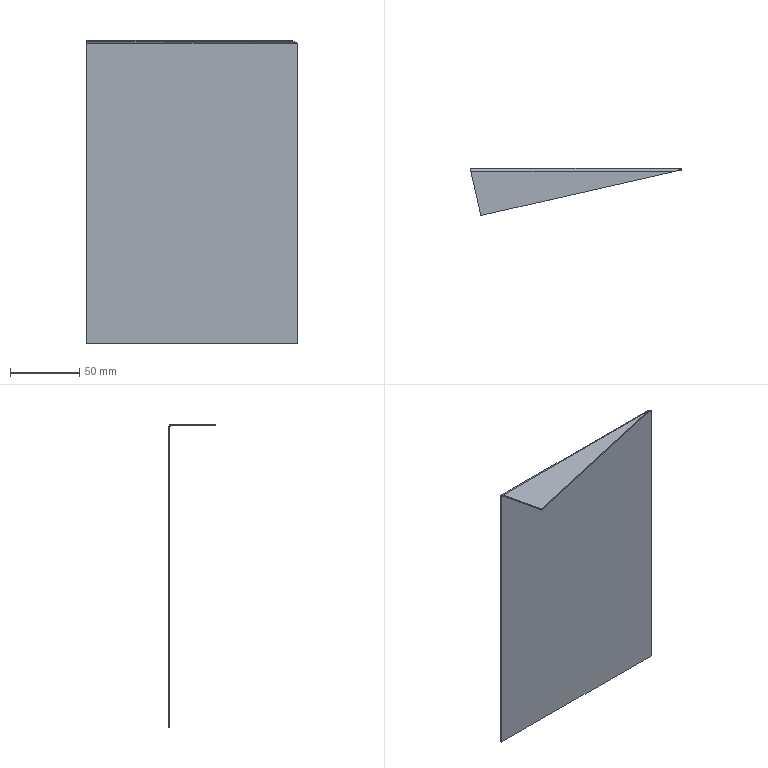Part | 1 solid | 13 faces | box 152.5 x 34 x 219 mm | volume 35812 mm3 | plane 9 | spline 2 | cylinder 2 | commonest cylinder face diameters 2 x1 4 x1
STEP:
#1=CARTESIAN_POINT('',(-152.5,-1.,107.5));
#2=VERTEX_POINT('',#1);
#3=CARTESIAN_POINT('',(0.,-1.,107.5));
#4=VERTEX_POINT('',#3);
#5=CARTESIAN_POINT('',(-152.5,-1.,107.5));
#6=DIRECTION('',(1.,0.,0.));
#7=VECTOR('',#6,1000.);
#8=LINE('',#5,#7);
#9=EDGE_CURVE('',#2,#4,#8,.T.);
#10=ORIENTED_EDGE('',*,*,#9,.F.);
#11=CARTESIAN_POINT('',(-152.5,-1.,-109.5));
#12=VERTEX_POINT('',#11);
#13=CARTESIAN_POINT('',(-152.5,-1.,109.5));
#14=DIRECTION('',(0.,0.,-1.));
#15=VECTOR('',#14,1000.);
#16=LINE('',#13,#15);
#17=EDGE_CURVE('',#2,#12,#16,.T.);
#18=ORIENTED_EDGE('',*,*,#17,.T.);
#19=CARTESIAN_POINT('',(0.,-1.,-109.5));
#20=VERTEX_POINT('',#19);
#21=CARTESIAN_POINT('',(-152.5,-1.,-109.5));
#22=DIRECTION('',(1.,0.,0.));
#23=VECTOR('',#22,1000.);
#24=LINE('',#21,#23);
#25=EDGE_CURVE('',#12,#20,#24,.T.);
#26=ORIENTED_EDGE('',*,*,#25,.T.);
#27=CARTESIAN_POINT('',(0.,-1.,109.5));
#28=DIRECTION('',(0.,0.,-1.));
#29=VECTOR('',#28,1000.);
#30=LINE('',#27,#29);
#31=EDGE_CURVE('',#4,#20,#30,.T.);
#32=ORIENTED_EDGE('',*,*,#31,.F.);
#33=EDGE_LOOP('',(#10,#18,#26,#32));
#34=FACE_OUTER_BOUND('',#33,.T.);
#35=CARTESIAN_POINT('',(-152.5,-1.,109.5));
#36=DIRECTION('',(0.,1.,0.));
#37=DIRECTION('',(0.,0.,1.));
#38=AXIS2_PLACEMENT_3D('',#35,#36,#37);
#39=PLANE('',#38);
#40=ADVANCED_FACE('',(#34),#39,.F.);
#41=CARTESIAN_POINT('',(-152.5,0.,107.5));
#42=VERTEX_POINT('',#41);
#43=CARTESIAN_POINT('',(-152.5,0.,-109.5));
#44=VERTEX_POINT('',#43);
#45=CARTESIAN_POINT('',(-152.5,0.,109.5));
#46=DIRECTION('',(0.,0.,-1.));
#47=VECTOR('',#46,1000.);
#48=LINE('',#45,#47);
#49=EDGE_CURVE('',#42,#44,#48,.T.);
#50=ORIENTED_EDGE('',*,*,#49,.F.);
#51=CARTESIAN_POINT('',(0.,0.,107.5));
#52=VERTEX_POINT('',#51);
#53=CARTESIAN_POINT('',(-152.5,0.,107.5));
#54=DIRECTION('',(1.,0.,0.));
#55=VECTOR('',#54,1000.);
#56=LINE('',#53,#55);
#57=EDGE_CURVE('',#42,#52,#56,.T.);
#58=ORIENTED_EDGE('',*,*,#57,.T.);
#59=CARTESIAN_POINT('',(0.,0.,-109.5));
#60=VERTEX_POINT('',#59);
#61=CARTESIAN_POINT('',(0.,0.,109.5));
#62=DIRECTION('',(0.,0.,-1.));
#63=VECTOR('',#62,1000.);
#64=LINE('',#61,#63);
#65=EDGE_CURVE('',#52,#60,#64,.T.);
#66=ORIENTED_EDGE('',*,*,#65,.T.);
#67=CARTESIAN_POINT('',(-152.5,0.,-109.5));
#68=DIRECTION('',(1.,0.,0.));
#69=VECTOR('',#68,1000.);
#70=LINE('',#67,#69);
#71=EDGE_CURVE('',#44,#60,#70,.T.);
#72=ORIENTED_EDGE('',*,*,#71,.F.);
#73=EDGE_LOOP('',(#50,#58,#66,#72));
#74=FACE_OUTER_BOUND('',#73,.T.);
#75=CARTESIAN_POINT('',(-152.5,0.,109.5));
#76=DIRECTION('',(0.,1.,0.));
#77=DIRECTION('',(0.,0.,1.));
#78=AXIS2_PLACEMENT_3D('',#75,#76,#77);
#79=PLANE('',#78);
#80=ADVANCED_FACE('',(#74),#79,.T.);
#81=ORIENTED_EDGE('',*,*,#17,.F.);
#82=CARTESIAN_POINT('',(-152.5,-1.,107.5));
#83=DIRECTION('',(0.,1.,0.));
#84=VECTOR('',#83,1000.);
#85=LINE('',#82,#84);
#86=EDGE_CURVE('',#2,#42,#85,.T.);
#87=ORIENTED_EDGE('',*,*,#86,.T.);
#88=ORIENTED_EDGE('',*,*,#49,.T.);
#89=CARTESIAN_POINT('',(-152.5,-1.,-109.5));
#90=DIRECTION('',(0.,1.,0.));
#91=VECTOR('',#90,1000.);
#92=LINE('',#89,#91);
#93=EDGE_CURVE('',#12,#44,#92,.T.);
#94=ORIENTED_EDGE('',*,*,#93,.F.);
#95=EDGE_LOOP('',(#81,#87,#88,#94));
#96=FACE_OUTER_BOUND('',#95,.T.);
#97=CARTESIAN_POINT('',(-152.5,-1.,109.5));
#98=DIRECTION('',(-1.,0.,0.));
#99=DIRECTION('',(0.,0.,1.));
#100=AXIS2_PLACEMENT_3D('',#97,#98,#99);
#101=PLANE('',#100);
#102=ADVANCED_FACE('',(#96),#101,.T.);
#103=CARTESIAN_POINT('',(0.,-1.,107.5));
#104=DIRECTION('',(0.,1.,0.));
#105=VECTOR('',#104,1000.);
#106=LINE('',#103,#105);
#107=EDGE_CURVE('',#4,#52,#106,.T.);
#108=ORIENTED_EDGE('',*,*,#107,.F.);
#109=ORIENTED_EDGE('',*,*,#31,.T.);
#110=CARTESIAN_POINT('',(0.,0.,-109.5));
#111=DIRECTION('',(0.,-1.,0.));
#112=VECTOR('',#111,1000.);
#113=LINE('',#110,#112);
#114=EDGE_CURVE('',#60,#20,#113,.T.);
#115=ORIENTED_EDGE('',*,*,#114,.F.);
#116=ORIENTED_EDGE('',*,*,#65,.F.);
#117=EDGE_LOOP('',(#108,#109,#115,#116));
#118=FACE_OUTER_BOUND('',#117,.T.);
#119=CARTESIAN_POINT('',(0.,0.,109.5));
#120=DIRECTION('',(1.,0.,0.));
#121=DIRECTION('',(0.,0.,-1.));
#122=AXIS2_PLACEMENT_3D('',#119,#120,#121);
#123=PLANE('',#122);
#124=ADVANCED_FACE('',(#118),#123,.T.);
#125=ORIENTED_EDGE('',*,*,#25,.F.);
#126=ORIENTED_EDGE('',*,*,#93,.T.);
#127=ORIENTED_EDGE('',*,*,#71,.T.);
#128=ORIENTED_EDGE('',*,*,#114,.T.);
#129=EDGE_LOOP('',(#125,#126,#127,#128));
#130=FACE_OUTER_BOUND('',#129,.T.);
#131=CARTESIAN_POINT('',(0.,0.,-109.5));
#132=DIRECTION('',(0.,0.,-1.));
#133=DIRECTION('',(-1.,0.,0.));
#134=AXIS2_PLACEMENT_3D('',#131,#132,#133);
#135=PLANE('',#134);
#136=ADVANCED_FACE('',(#130),#135,.T.);
#137=CARTESIAN_POINT('',(-4.394,-2.,108.5));
#138=VERTEX_POINT('',#137);
#139=CARTESIAN_POINT('',(-4.394,-2.,109.5));
#140=VERTEX_POINT('',#139);
#141=CARTESIAN_POINT('',(-4.394,-2.,109.5));
#142=DIRECTION('',(0.,0.,1.));
#143=VECTOR('',#142,1000.);
#144=LINE('',#141,#143);
#145=EDGE_CURVE('',#138,#140,#144,.T.);
#146=ORIENTED_EDGE('',*,*,#145,.F.);
#147=CARTESIAN_POINT('',(0.,-1.,107.5));
#148=CARTESIAN_POINT('',(-0.3672,-1.,107.631));
#149=CARTESIAN_POINT('',(-0.7317,-1.026,107.762));
#150=CARTESIAN_POINT('',(-1.462,-1.126,108.003));
#151=CARTESIAN_POINT('',(-1.828,-1.2,108.114));
#152=CARTESIAN_POINT('',(-2.561,-1.385,108.299));
#153=CARTESIAN_POINT('',(-2.928,-1.496,108.374));
#154=CARTESIAN_POINT('',(-3.661,-1.738,108.474));
#155=CARTESIAN_POINT('',(-4.026,-1.869,108.5));
#156=CARTESIAN_POINT('',(-4.394,-2.,108.5));
#157=B_SPLINE_CURVE_WITH_KNOTS('',3,(#147,#148,#149,#150,#151,#152,#153,#154,#155,#156),.UNSPECIFIED.,.F.,.F.,(4,2,2,2,4),(0.,0.001162,0.002325,0.003487,0.00465),.UNSPECIFIED.);
#158=EDGE_CURVE('',#4,#138,#157,.T.);
#159=ORIENTED_EDGE('',*,*,#158,.F.);
#160=ORIENTED_EDGE('',*,*,#107,.T.);
#161=CARTESIAN_POINT('',(0.,0.,107.5));
#162=CARTESIAN_POINT('',(-0.3691,0.,107.764));
#163=CARTESIAN_POINT('',(-0.7313,-0.052,108.023));
#164=CARTESIAN_POINT('',(-1.46,-0.2511,108.505));
#165=CARTESIAN_POINT('',(-1.831,-0.4008,108.729));
#166=CARTESIAN_POINT('',(-2.56,-0.7691,109.098));
#167=CARTESIAN_POINT('',(-2.923,-0.9887,109.246));
#168=CARTESIAN_POINT('',(-3.66,-1.476,109.448));
#169=CARTESIAN_POINT('',(-4.024,-1.736,109.5));
#170=CARTESIAN_POINT('',(-4.394,-2.,109.5));
#171=B_SPLINE_CURVE_WITH_KNOTS('',3,(#161,#162,#163,#164,#165,#166,#167,#168,#169,#170),.UNSPECIFIED.,.F.,.F.,(4,2,2,2,4),(0.,0.001342,0.002685,0.004027,0.005369),.UNSPECIFIED.);
#172=EDGE_CURVE('',#52,#140,#171,.T.);
#173=ORIENTED_EDGE('',*,*,#172,.T.);
#174=EDGE_LOOP('',(#146,#159,#160,#173));
#175=FACE_OUTER_BOUND('',#174,.T.);
#176=CARTESIAN_POINT('',(0.,0.01,107.5));
#177=CARTESIAN_POINT('',(-0.3662,0.01,107.763));
#178=CARTESIAN_POINT('',(-0.7323,-0.04231,108.026));
#179=CARTESIAN_POINT('',(-1.465,-0.2437,108.512));
#180=CARTESIAN_POINT('',(-1.831,-0.3927,108.735));
#181=CARTESIAN_POINT('',(-2.563,-0.7648,109.107));
#182=CARTESIAN_POINT('',(-2.929,-0.9877,109.256));
#183=CARTESIAN_POINT('',(-3.661,-1.474,109.458));
#184=CARTESIAN_POINT('',(-4.027,-1.737,109.51));
#185=CARTESIAN_POINT('',(-4.394,-2.,109.51));
#186=CARTESIAN_POINT('',(0.,0.,107.5));
#187=CARTESIAN_POINT('',(-0.3662,0.,107.762));
#188=CARTESIAN_POINT('',(-0.7323,-0.05205,108.023));
#189=CARTESIAN_POINT('',(-1.465,-0.2524,108.507));
#190=CARTESIAN_POINT('',(-1.831,-0.4007,108.729));
#191=CARTESIAN_POINT('',(-2.563,-0.7709,109.099));
#192=CARTESIAN_POINT('',(-2.929,-0.9928,109.248));
#193=CARTESIAN_POINT('',(-3.661,-1.477,109.448));
#194=CARTESIAN_POINT('',(-4.027,-1.738,109.5));
#195=CARTESIAN_POINT('',(-4.394,-2.,109.5));
#196=CARTESIAN_POINT('',(0.,-1.,107.5));
#197=CARTESIAN_POINT('',(-0.3661,-1.,107.631));
#198=CARTESIAN_POINT('',(-0.7323,-1.026,107.762));
#199=CARTESIAN_POINT('',(-1.465,-1.126,108.004));
#200=CARTESIAN_POINT('',(-1.831,-1.2,108.115));
#201=CARTESIAN_POINT('',(-2.563,-1.385,108.3));
#202=CARTESIAN_POINT('',(-2.929,-1.496,108.374));
#203=CARTESIAN_POINT('',(-3.661,-1.738,108.474));
#204=CARTESIAN_POINT('',(-4.027,-1.869,108.5));
#205=CARTESIAN_POINT('',(-4.394,-2.,108.5));
#206=CARTESIAN_POINT('',(0.,-1.01,107.5));
#207=CARTESIAN_POINT('',(-0.3661,-1.01,107.63));
#208=CARTESIAN_POINT('',(-0.7323,-1.036,107.759));
#209=CARTESIAN_POINT('',(-1.465,-1.135,107.999));
#210=CARTESIAN_POINT('',(-1.831,-1.208,108.108));
#211=CARTESIAN_POINT('',(-2.563,-1.392,108.292));
#212=CARTESIAN_POINT('',(-2.929,-1.501,108.365));
#213=CARTESIAN_POINT('',(-3.661,-1.741,108.464));
#214=CARTESIAN_POINT('',(-4.027,-1.87,108.49));
#215=CARTESIAN_POINT('',(-4.394,-2.,108.49));
#216=B_SPLINE_SURFACE_WITH_KNOTS('',1,3,((#176,#177,#178,#179,#180,#181,#182,#183,#184,#185),(#186,#187,#188,#189,#190,#191,#192,#193,#194,#195),(#196,#197,#198,#199,#200,#201,#202,#203,#204,#205),(#206,#207,#208,#209,#210,#211,#212,#213,#214,#215)),.UNSPECIFIED.,.F.,.F.,.F.,(2,1,1,2),(4,2,2,2,4),(-0.01,0.,1.,1.01),(0.,0.25,0.5,0.75,1.),.UNSPECIFIED.);
#217=ADVANCED_FACE('',(#175),#216,.F.);
#218=CARTESIAN_POINT('',(-152.272,-2.,108.5));
#219=VERTEX_POINT('',#218);
#220=CARTESIAN_POINT('',(-152.272,-2.,108.5));
#221=CARTESIAN_POINT('',(-152.31,-1.738,108.5));
#222=CARTESIAN_POINT('',(-152.348,-1.478,108.392));
#223=CARTESIAN_POINT('',(-152.424,-1.108,108.022));
#224=CARTESIAN_POINT('',(-152.462,-1.,107.762));
#225=CARTESIAN_POINT('',(-152.5,-1.,107.5));
#226=B_SPLINE_CURVE_WITH_KNOTS('',3,(#220,#221,#222,#223,#224,#225),.UNSPECIFIED.,.F.,.F.,(4,2,4),(0.,0.5,1.),.UNSPECIFIED.);
#227=EDGE_CURVE('',#219,#2,#226,.T.);
#228=ORIENTED_EDGE('',*,*,#227,.F.);
#229=CARTESIAN_POINT('',(-152.272,-2.,109.5));
#230=VERTEX_POINT('',#229);
#231=CARTESIAN_POINT('',(-152.272,-2.,108.5));
#232=DIRECTION('',(0.,0.,1.));
#233=VECTOR('',#232,1000.);
#234=LINE('',#231,#233);
#235=EDGE_CURVE('',#219,#230,#234,.T.);
#236=ORIENTED_EDGE('',*,*,#235,.T.);
#237=CARTESIAN_POINT('',(-152.272,-2.,109.5));
#238=CARTESIAN_POINT('',(-152.291,-1.738,109.5));
#239=CARTESIAN_POINT('',(-152.31,-1.477,109.448));
#240=CARTESIAN_POINT('',(-152.348,-0.9928,109.248));
#241=CARTESIAN_POINT('',(-152.367,-0.7709,109.099));
#242=CARTESIAN_POINT('',(-152.405,-0.4007,108.729));
#243=CARTESIAN_POINT('',(-152.424,-0.2524,108.507));
#244=CARTESIAN_POINT('',(-152.462,-0.05205,108.023));
#245=CARTESIAN_POINT('',(-152.481,0.,107.762));
#246=CARTESIAN_POINT('',(-152.5,0.,107.5));
#247=B_SPLINE_CURVE_WITH_KNOTS('',3,(#237,#238,#239,#240,#241,#242,#243,#244,#245,#246),.UNSPECIFIED.,.F.,.F.,(4,2,2,2,4),(0.,0.25,0.5,0.75,1.),.UNSPECIFIED.);
#248=EDGE_CURVE('',#230,#42,#247,.T.);
#249=ORIENTED_EDGE('',*,*,#248,.T.);
#250=ORIENTED_EDGE('',*,*,#86,.F.);
#251=EDGE_LOOP('',(#228,#236,#249,#250));
#252=FACE_OUTER_BOUND('',#251,.T.);
#253=CARTESIAN_POINT('',(-152.272,-2.,109.51));
#254=CARTESIAN_POINT('',(-152.291,-1.737,109.51));
#255=CARTESIAN_POINT('',(-152.31,-1.474,109.458));
#256=CARTESIAN_POINT('',(-152.348,-0.9877,109.256));
#257=CARTESIAN_POINT('',(-152.367,-0.7648,109.107));
#258=CARTESIAN_POINT('',(-152.405,-0.3927,108.735));
#259=CARTESIAN_POINT('',(-152.424,-0.2437,108.512));
#260=CARTESIAN_POINT('',(-152.462,-0.04231,108.026));
#261=CARTESIAN_POINT('',(-152.481,0.01,107.763));
#262=CARTESIAN_POINT('',(-152.5,0.01,107.5));
#263=CARTESIAN_POINT('',(-152.272,-2.,109.5));
#264=CARTESIAN_POINT('',(-152.291,-1.738,109.5));
#265=CARTESIAN_POINT('',(-152.31,-1.477,109.448));
#266=CARTESIAN_POINT('',(-152.348,-0.9928,109.248));
#267=CARTESIAN_POINT('',(-152.367,-0.7709,109.099));
#268=CARTESIAN_POINT('',(-152.405,-0.4007,108.729));
#269=CARTESIAN_POINT('',(-152.424,-0.2524,108.507));
#270=CARTESIAN_POINT('',(-152.462,-0.05205,108.023));
#271=CARTESIAN_POINT('',(-152.481,0.,107.762));
#272=CARTESIAN_POINT('',(-152.5,0.,107.5));
#273=CARTESIAN_POINT('',(-152.272,-2.,108.5));
#274=CARTESIAN_POINT('',(-152.291,-1.869,108.5));
#275=CARTESIAN_POINT('',(-152.31,-1.738,108.474));
#276=CARTESIAN_POINT('',(-152.348,-1.496,108.374));
#277=CARTESIAN_POINT('',(-152.367,-1.385,108.3));
#278=CARTESIAN_POINT('',(-152.405,-1.2,108.115));
#279=CARTESIAN_POINT('',(-152.424,-1.126,108.004));
#280=CARTESIAN_POINT('',(-152.462,-1.026,107.762));
#281=CARTESIAN_POINT('',(-152.481,-1.,107.631));
#282=CARTESIAN_POINT('',(-152.5,-1.,107.5));
#283=CARTESIAN_POINT('',(-152.272,-2.,108.49));
#284=CARTESIAN_POINT('',(-152.291,-1.87,108.49));
#285=CARTESIAN_POINT('',(-152.31,-1.741,108.464));
#286=CARTESIAN_POINT('',(-152.348,-1.501,108.365));
#287=CARTESIAN_POINT('',(-152.367,-1.392,108.292));
#288=CARTESIAN_POINT('',(-152.405,-1.208,108.108));
#289=CARTESIAN_POINT('',(-152.424,-1.135,107.999));
#290=CARTESIAN_POINT('',(-152.462,-1.036,107.759));
#291=CARTESIAN_POINT('',(-152.481,-1.01,107.63));
#292=CARTESIAN_POINT('',(-152.5,-1.01,107.5));
#293=B_SPLINE_SURFACE_WITH_KNOTS('',1,3,((#253,#254,#255,#256,#257,#258,#259,#260,#261,#262),(#263,#264,#265,#266,#267,#268,#269,#270,#271,#272),(#273,#274,#275,#276,#277,#278,#279,#280,#281,#282),(#283,#284,#285,#286,#287,#288,#289,#290,#291,#292)),.UNSPECIFIED.,.F.,.F.,.F.,(2,1,1,2),(4,2,2,2,4),(-0.01,0.,1.,1.01),(0.,0.25,0.5,0.75,1.),.UNSPECIFIED.);
#294=ADVANCED_FACE('',(#252),#293,.F.);
#295=ORIENTED_EDGE('',*,*,#57,.F.);
#296=ORIENTED_EDGE('',*,*,#248,.F.);
#297=CARTESIAN_POINT('',(0.,-2.,109.5));
#298=DIRECTION('',(-1.,0.,0.));
#299=VECTOR('',#298,1000.);
#300=LINE('',#297,#299);
#301=EDGE_CURVE('',#140,#230,#300,.T.);
#302=ORIENTED_EDGE('',*,*,#301,.F.);
#303=ORIENTED_EDGE('',*,*,#172,.F.);
#304=EDGE_LOOP('',(#295,#296,#302,#303));
#305=FACE_OUTER_BOUND('',#304,.T.);
#306=CARTESIAN_POINT('',(-152.5,-2.,107.5));
#307=DIRECTION('',(-1.,0.,0.));
#308=DIRECTION('',(0.,0.,1.));
#309=AXIS2_PLACEMENT_3D('',#306,#307,#308);
#310=CYLINDRICAL_SURFACE('',#309,2.);
#311=ADVANCED_FACE('',(#305),#310,.T.);
#312=ORIENTED_EDGE('',*,*,#9,.T.);
#313=ORIENTED_EDGE('',*,*,#158,.T.);
#314=CARTESIAN_POINT('',(-4.394,-2.,108.5));
#315=DIRECTION('',(-1.,0.,0.));
#316=VECTOR('',#315,1000.);
#317=LINE('',#314,#316);
#318=EDGE_CURVE('',#138,#219,#317,.T.);
#319=ORIENTED_EDGE('',*,*,#318,.T.);
#320=ORIENTED_EDGE('',*,*,#227,.T.);
#321=EDGE_LOOP('',(#312,#313,#319,#320));
#322=FACE_OUTER_BOUND('',#321,.T.);
#323=CARTESIAN_POINT('',(-152.5,-2.,107.5));
#324=DIRECTION('',(-1.,0.,0.));
#325=DIRECTION('',(0.,0.,1.));
#326=AXIS2_PLACEMENT_3D('',#323,#324,#325);
#327=CYLINDRICAL_SURFACE('',#326,1.);
#328=ADVANCED_FACE('',(#322),#327,.F.);
#329=ORIENTED_EDGE('',*,*,#235,.F.);
#330=CARTESIAN_POINT('',(-144.989,-34.,108.5));
#331=VERTEX_POINT('',#330);
#332=CARTESIAN_POINT('',(-144.989,-34.,108.5));
#333=DIRECTION('',(0.2219,-0.9751,0.));
#334=VECTOR('',#333,1000.);
#335=LINE('',#332,#334);
#336=EDGE_CURVE('',#219,#331,#335,.T.);
#337=ORIENTED_EDGE('',*,*,#336,.T.);
#338=CARTESIAN_POINT('',(-144.989,-34.,109.5));
#339=VERTEX_POINT('',#338);
#340=CARTESIAN_POINT('',(-144.989,-34.,109.5));
#341=DIRECTION('',(0.,0.,-1.));
#342=VECTOR('',#341,1000.);
#343=LINE('',#340,#342);
#344=EDGE_CURVE('',#339,#331,#343,.T.);
#345=ORIENTED_EDGE('',*,*,#344,.F.);
#346=CARTESIAN_POINT('',(-145.205,-33.049,109.5));
#347=DIRECTION('',(0.2219,-0.9751,0.));
#348=VECTOR('',#347,1000.);
#349=LINE('',#346,#348);
#350=EDGE_CURVE('',#230,#339,#349,.T.);
#351=ORIENTED_EDGE('',*,*,#350,.F.);
#352=EDGE_LOOP('',(#329,#337,#345,#351));
#353=FACE_OUTER_BOUND('',#352,.T.);
#354=CARTESIAN_POINT('',(-144.989,-34.,109.5));
#355=DIRECTION('',(0.9751,0.2219,0.));
#356=DIRECTION('',(-0.2219,0.9751,0.));
#357=AXIS2_PLACEMENT_3D('',#354,#355,#356);
#358=PLANE('',#357);
#359=ADVANCED_FACE('',(#353),#358,.F.);
#360=ORIENTED_EDGE('',*,*,#145,.T.);
#361=CARTESIAN_POINT('',(0.2164,-0.9507,109.5));
#362=DIRECTION('',(0.9751,0.2219,0.));
#363=VECTOR('',#362,1000.);
#364=LINE('',#361,#363);
#365=EDGE_CURVE('',#339,#140,#364,.T.);
#366=ORIENTED_EDGE('',*,*,#365,.F.);
#367=ORIENTED_EDGE('',*,*,#344,.T.);
#368=CARTESIAN_POINT('',(0.,-1.,108.5));
#369=DIRECTION('',(0.9751,0.2219,0.));
#370=VECTOR('',#369,1000.);
#371=LINE('',#368,#370);
#372=EDGE_CURVE('',#331,#138,#371,.T.);
#373=ORIENTED_EDGE('',*,*,#372,.T.);
#374=EDGE_LOOP('',(#360,#366,#367,#373));
#375=FACE_OUTER_BOUND('',#374,.T.);
#376=CARTESIAN_POINT('',(0.,-1.,109.5));
#377=DIRECTION('',(-0.2219,0.9751,0.));
#378=DIRECTION('',(-0.9751,-0.2219,0.));
#379=AXIS2_PLACEMENT_3D('',#376,#377,#378);
#380=PLANE('',#379);
#381=ADVANCED_FACE('',(#375),#380,.F.);
#382=ORIENTED_EDGE('',*,*,#365,.T.);
#383=ORIENTED_EDGE('',*,*,#301,.T.);
#384=ORIENTED_EDGE('',*,*,#350,.T.);
#385=EDGE_LOOP('',(#382,#383,#384));
#386=FACE_OUTER_BOUND('',#385,.T.);
#387=CARTESIAN_POINT('',(0.,0.,109.5));
#388=DIRECTION('',(0.,0.,1.));
#389=DIRECTION('',(0.,-1.,0.));
#390=AXIS2_PLACEMENT_3D('',#387,#388,#389);
#391=PLANE('',#390);
#392=ADVANCED_FACE('',(#386),#391,.T.);
#393=ORIENTED_EDGE('',*,*,#318,.F.);
#394=ORIENTED_EDGE('',*,*,#372,.F.);
#395=ORIENTED_EDGE('',*,*,#336,.F.);
#396=EDGE_LOOP('',(#393,#394,#395));
#397=FACE_OUTER_BOUND('',#396,.T.);
#398=CARTESIAN_POINT('',(0.,0.,108.5));
#399=DIRECTION('',(0.,0.,1.));
#400=DIRECTION('',(0.,-1.,0.));
#401=AXIS2_PLACEMENT_3D('',#398,#399,#400);
#402=PLANE('',#401);
#403=ADVANCED_FACE('',(#397),#402,.F.);
#404=CLOSED_SHELL('',(#40,#80,#102,#124,#136,#217,#294,#311,#328,#359,#381,#392,#403));
#405=MANIFOLD_SOLID_BREP('',#404);
#406=CARTESIAN_POINT('',(0.,0.,0.));
#407=DIRECTION('',(0.,0.,1.));
#408=DIRECTION('',(1.,0.,0.));
#409=AXIS2_PLACEMENT_3D('',#406,#407,#408);
#410=(LENGTH_UNIT()NAMED_UNIT(*)SI_UNIT(.MILLI.,.METRE.));
#411=UNCERTAINTY_MEASURE_WITH_UNIT(LENGTH_MEASURE(0.00001),#410,'','');
#412=(NAMED_UNIT(*)PLANE_ANGLE_UNIT()SI_UNIT($,.RADIAN.));
#413=(NAMED_UNIT(*)SI_UNIT($,.STERADIAN.)SOLID_ANGLE_UNIT());
#414=(GEOMETRIC_REPRESENTATION_CONTEXT(3)GLOBAL_UNCERTAINTY_ASSIGNED_CONTEXT((#411))GLOBAL_UNIT_ASSIGNED_CONTEXT((#410,#412,#413))REPRESENTATION_CONTEXT('',''));
#415=ADVANCED_BREP_SHAPE_REPRESENTATION('',(#405,#409),#414);